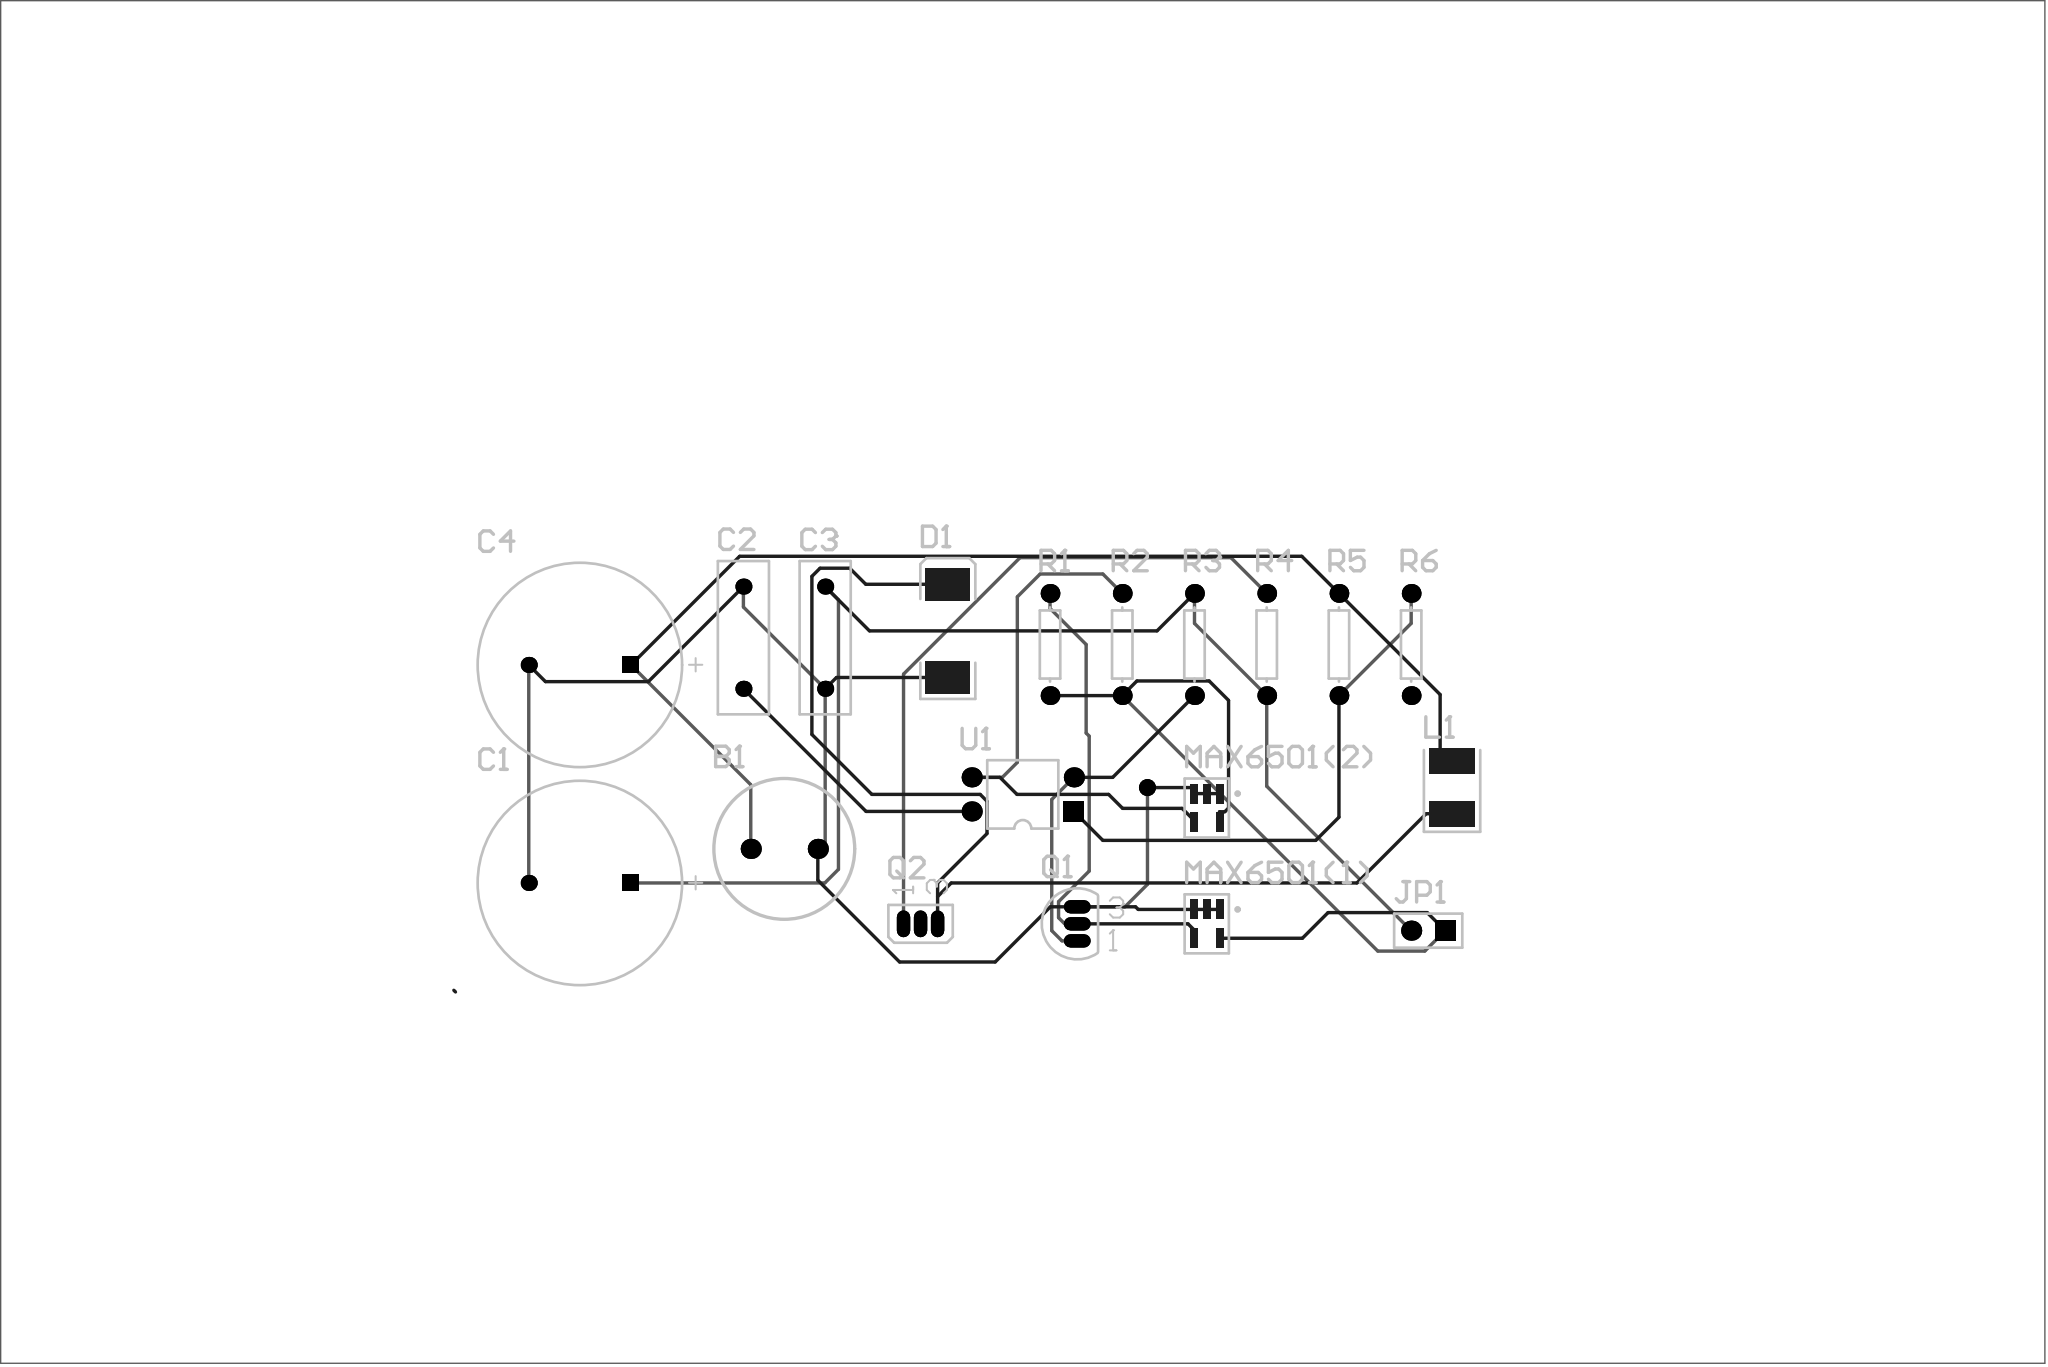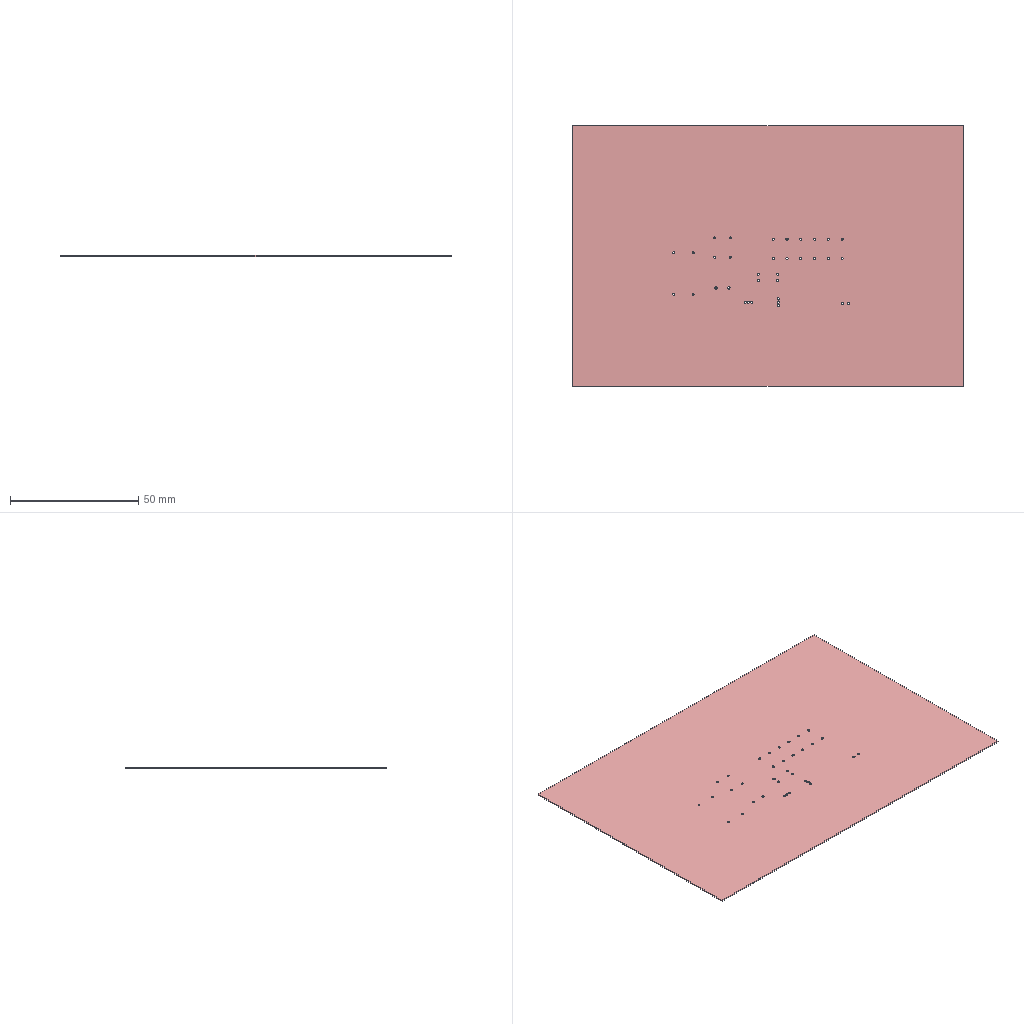Circuit board layout | Cadence Allegro | box 152.4 x 101.6 x 0.4 mm
Layer stack:
# Altium Designer layer stack of  (unit mm; dielectric type: 0 none, 1 core, 2 prepreg, 3 surface material)
index,name,kind,layer,copper_thickness_mm,dielectric_type,dielectric_thickness_mm,dielectric_material,dielectric_constant
0,Top Paste,other,,,,,,
1,Top Overlay,other,,,,,,
2,Top Solder,dielectric,,,3,0.0102,Solder Resist,3.5
3,Top Layer,copper,Top Layer,0.0356,,,,
4,Dielectric1,dielectric,,,0,0.32,FR-4,4.8
5,Bottom Layer,copper,Bottom Layer,0.0356,,,,
6,Bottom Solder,dielectric,,,3,0.0102,Solder Resist,3.5
7,Bottom Overlay,other,,,,,,
8,Bottom Paste,other,,,,,,
# drill layer pairs: low layer,high layer
drill_pair,Top Layer,Bottom Layer
Part placement:
Designator,Comment,Layer,Footprint,Center-X(mm),Center-Y(mm),Rotation
B1,Motor,TopLayer,RB5-10.5,68.072,97.028,0
C1,Cap Pol1,TopLayer,RB7.6-15,52.832,94.488,0
C2,Cap,TopLayer,RAD-0.3,65.024,112.776,270
C3,Cap,TopLayer,RAD-0.3,71.12,112.776,90
C4,Cap Pol1,TopLayer,RB7.6-15,52.832,110.744,0
D1,Diode,TopLayer,DSO-C2/X3.3,80.264,113.284,90
JP1,Header 2,TopLayer,HDR1X2,116.078,90.932,180
L1,Inductor,TopLayer,CC4532-1812,117.856,101.6,90
MAX6501(1),MAX6501,TopLayer,SO-G5/P.95,99.568,91.44,180
MAX6501(2),MAX6501,TopLayer,SO-G5/P.95,99.568,100.076,180
Q1,NPN,TopLayer,BCY-W3,89.916,91.44,0
Q2,IRF7416,TopLayer,BCY-W3/H.8,78.232,91.44,90
R1,Res1,TopLayer,AXIAL-0.3,87.884,112.268,90
R2,Res1,TopLayer,AXIAL-0.3,93.269,112.268,90
R3,Res1,TopLayer,AXIAL-0.3,98.654,112.268,90
R4,Res1,TopLayer,AXIAL-0.3,104.038,112.268,90
R5,Res1,TopLayer,AXIAL-0.3,109.423,112.268,90
R6,Res1,TopLayer,AXIAL-0.3,114.808,112.268,90
U1,MAX1626,TopLayer,DIP-4,85.852,101.092,90
Pad and via stacks:
# Altium Designer via and pad stacks of  (unit mm). Each distinct definition once, with the count of objects using it.
# via: kind,start_layer,end_layer,hole_mm,diameter_mm,mode(0 simple;1 top-mid-bottom;2 full stack),diameter_per_layer,count,example_net
# pad: kind,layer,hole_mm,hole_type(0 round;1 square;2 slot),plating,top_size,top_shape(1 round;2 rect;3 octagon;9 rounded rect),mid_size,bottom_size,mode,footprint,size_per_layer,count,example
pad,Top Layer,0,0,plated,0.55x1.45,2,0.55x1.45,0.55x1.45,0,SO-G5/P.95,,10,MAX6501(2).5
pad,Top Layer,0,0,plated,2.4x3.3,2,2.4x3.3,2.4x3.3,0,DSO-C2/X3.3,,2,D1.1
pad,Top Layer,0,0,plated,1.9x3.4,2,1.9x3.4,1.9x3.4,0,CC4532-1812,,2,L1.2
pad,Multi-Layer,0.85,0,plated,1.4x1.4,1,1.4x1.4,1.4x1.4,0,AXIAL-0.3,,12,R6.2
pad,Multi-Layer,0.9,0,plated,1.5x1.5,1,1.5x1.5,1.5x1.5,0,RB5-10.5,,2,B1.2
pad,Multi-Layer,0.7,0,plated,1.2x1.2,2,1.2x1.2,1.2x1.2,0,RB7.6-15,,2,C4.1
pad,Multi-Layer,0.7,0,plated,1.2x1.2,1,1.2x1.2,1.2x1.2,0,RB7.6-15,,2,C4.2
pad,Multi-Layer,0.7,0,plated,1.2x1.2,1,1.2x1.2,1.2x1.2,0,RAD-0.3,,4,C2.1
pad,Multi-Layer,0.8,0,plated,2x1,1,2x1,2x1,0,BCY-W3/H.8,,3,Q2.1
pad,Multi-Layer,0.9,0,plated,1.5x1.5,2,1.5x1.5,1.5x1.5,0,DIP-4,,1,U1.1
pad,Multi-Layer,0.9,0,plated,1.5x1.5,1,1.5x1.5,1.5x1.5,0,DIP-4,,3,U1.2
pad,Multi-Layer,0.9,0,plated,2x1,1,2x1,2x1,0,BCY-W3,,3,Q1.1
pad,Multi-Layer,0.9,0,plated,1.5x1.5,1,1.5x1.5,1.5x1.5,0,HDR1X2,,1,JP1.2
pad,Multi-Layer,0.9,0,plated,1.5x1.5,2,1.5x1.5,1.5x1.5,0,HDR1X2,,1,JP1.1
via,Top Layer,Bottom Layer,0.7112,1.27,0,,1,GND
Design rules, without the lines most boards share:
# Altium Designer design rules of  (exported by Altium Designer, unit mm)
# columns: name | kind | enabled | priority | scope1 | scope2 | descriptor | typed fields (field=value)
HoleToHoleClearance | 52 | enabled | 1 | All | All | Hole To Hole Clearance (Gap=10mil) (All),(All) | gap=0.254
DiffPairsRouting | 51 | enabled | 1 | All | All | Differential Pairs Uncoupled Length using the Gap Constraints (Min=10mil) (Max=10mil) (Prefered=10mil)  and Width Constraints (Min=15mil) (Max=15mil) (Prefered=15mil) (All) |
Testpoint | 43 | enabled | 1 | All | All | Fabrication Testpoint Style (Under Component=Yes) (All) |
TestPointUsage | 44 | enabled | 1 | All | All | Fabrication Testpoint Usage (Valid =One Required, Allow multiple per net=No) (All) |
SolderMaskExpansion | 13 | enabled | 1 | All | All | Solder Mask Expansion (Expansion =4mil) (All) | expansion=0.1016
PasteMaskExpansion | 14 | enabled | 1 | All | All | Paste Mask Expansion (Expansion =0mil) (All) | expansion=0
RoutingVias | 11 | enabled | 1 | All | All | Routing Via (MinHoleWidth=28mil) (MaxHoleWidth=28mil) (PreferredHoleWidth=28mil) (MinWidth=50mil) (MaxWidth=50mil) (PreferedWidth=50mil) (All) | via_min_hole=0.7112 via_max_hole=0.7112 via_preferred_diameter=1.27 via_preferred_hole=0.7112
Width | 2 | enabled | 1 | All | All | Width Constraint (Min=10mil) (Max=10mil) (Preferred=10mil) (All) |
PolygonConnect | 20 | enabled | 1 | All | All | Polygon Connect Rule(Relief Connect )(Conductor Width=10mil) (Relief Angle=90 Angle) (Entries=4) (Air Gap Width=10mil) (All),(All) | connect_style(0=relief,1=direct,2=none)=0 relief_conductor_width=0.254 relief_entries=4
PlaneConnect | 6 | enabled | 1 | All | All | Power Plane Connect Rule(Relief Connect )(Expansion=20mil) (Conductor Width=10mil) (Air Gap=10mil) (Entries=4) (All) | relief_conductor_width=0.254 relief_entries=4 relief_expansion=0.508
Clearance | 0 | enabled | 1 | All | All | Clearance Constraint (Gap=10mil) (All),(All) | gap=0.254